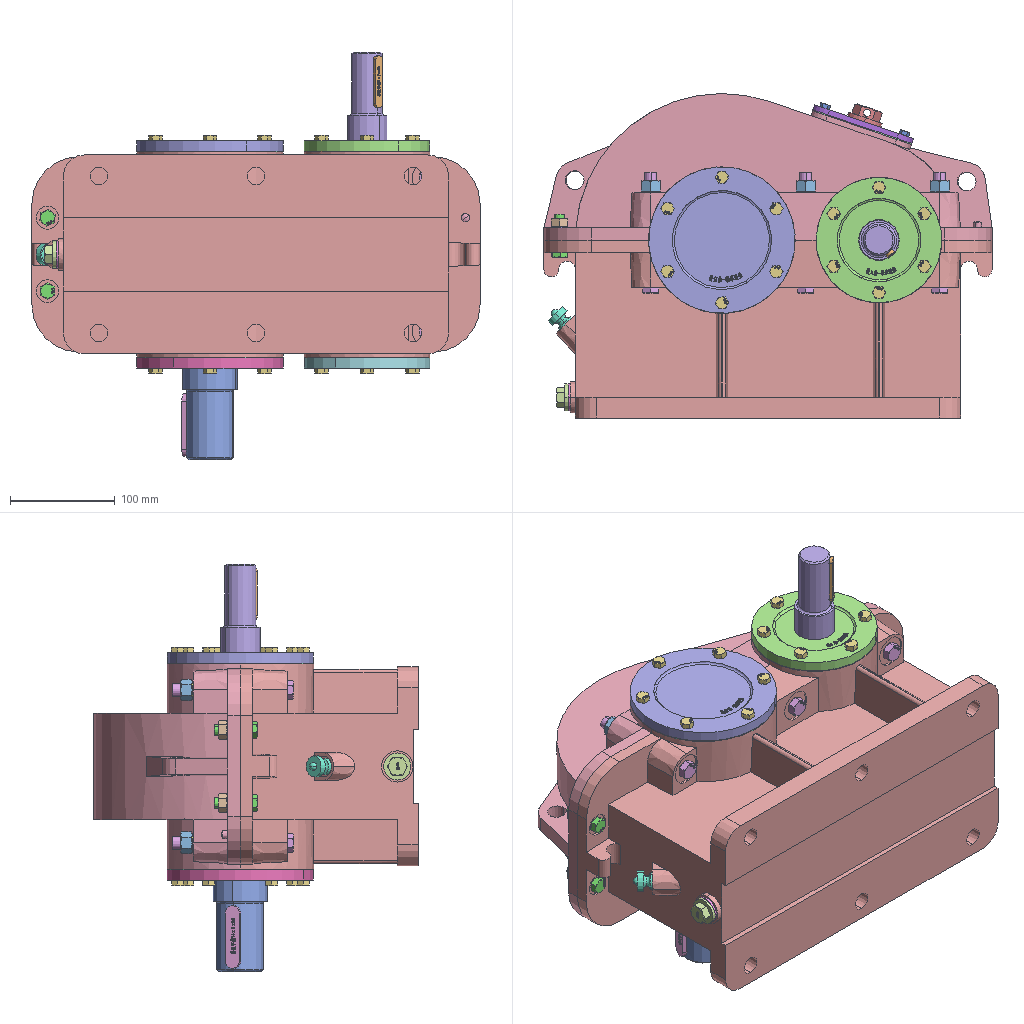Assembly | SolidWorks | 32 different items | 81 placed | box 428 x 310 x 389 mm
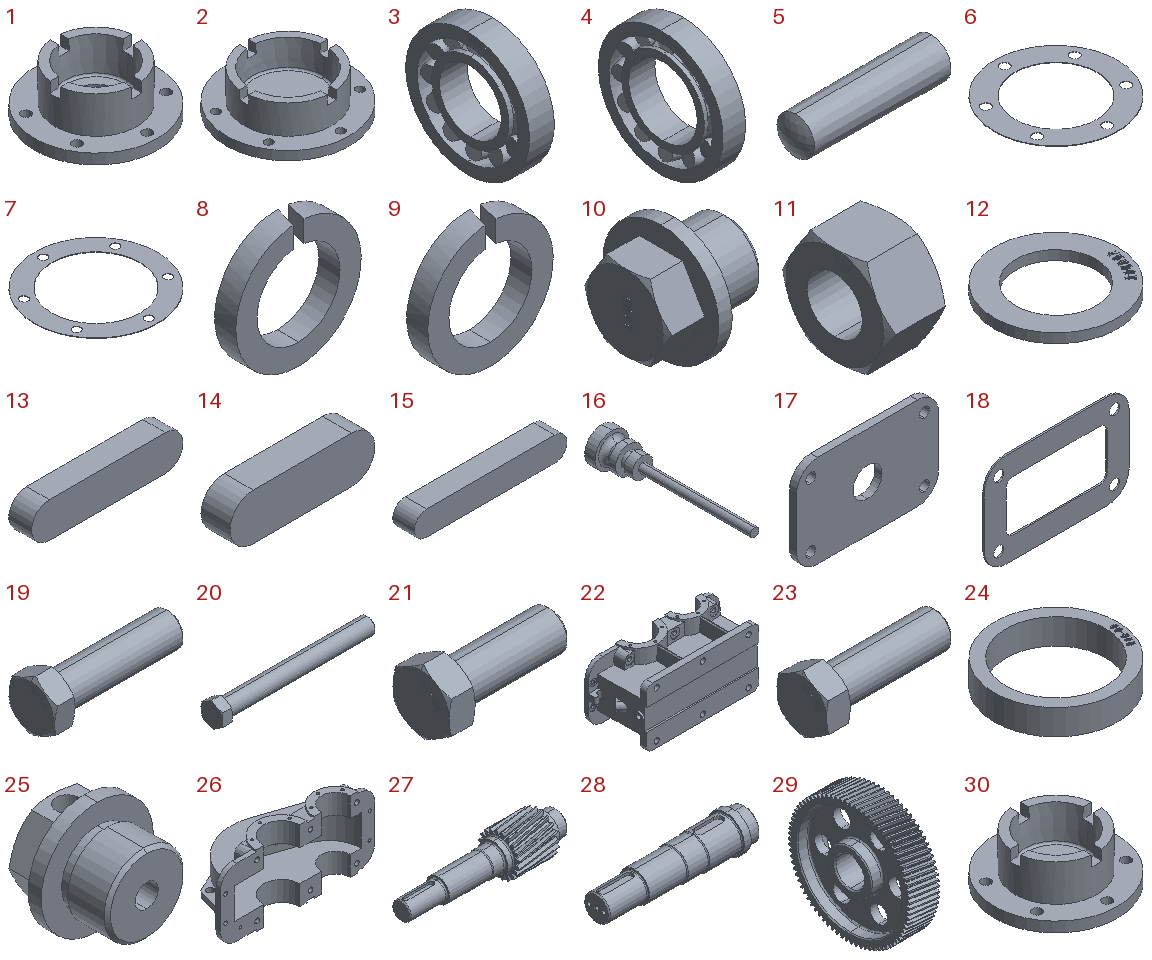Parts list (item | quantity | size | volume | features):
1 | x1 | 120 x 120 x 45.75 mm | 157075 mm3 | features ICE 6, CirPattern 2, Fillet 1, MirrorPattern 1, RevCut 1, Revolution 1
2 | x1 | 140 x 140 x 42.75 mm | 226052 mm3 | features ICE 5, CirPattern 2, Fillet 1, Revolution 1
3 | x2 | 19.75 x 80 x 80 mm | 48755 mm3 | features Revolution 5, CirPattern 1, ICE 1
4 | x2 | 22.75 x 100 x 100 mm | 79449 mm3 | features Revolution 5, CirPattern 1, ICE 1
5 | x2 | 30 x 8.048 x 8.048 mm | 1422 mm3 | features Revolution 1
6 | x2 | 120 x 120 x 0.5 mm | 2951 mm3 | features CirPattern 1, Extrusion 1, ICE 1
7 | x2 | 140 x 140 x 0.5 mm | 3579 mm3 | features CirPattern 1, Extrusion 1, ICE 1
8 | x2 | 15.4 x 2.6 x 15.4 mm | 262.555 mm3 | features ICE 2, Extrusion 1
9 | x6 | 18.4 x 3.1 x 18.4 mm | 446.274 mm3 | features ICE 2, Extrusion 1
10 | x1 | 23.1 x 26 x 26 mm | 5865 mm3 | features Chamfer 1, Extrusion 1, ICE 1, RevCut 1, Revolution 1
11 | x6 | 10.8 x 20.785 x 18 mm | 2135 mm3 | features 3DProfileFeature 1, Extrusion 1, HoleWzd 1, ICE 1, MirrorPattern 1, RevCut 1
12 | x1 | 26 x 26 x 2 mm | 607.665 mm3 | features Extrusion 1, ICE 1
13 | x1 | 60 x 9 x 14 mm | 7180 mm3 | features Extrusion 1, ICE 1
14 | x1 | 50 x 10 x 16 mm | 7451 mm3 | features Extrusion 1
15 | x1 | 50 x 7 x 8 mm | 2702 mm3 | features Extrusion 1, ICE 1
16 | x1 | 20 x 94 x 20 mm | 5502 mm3 | features Revolution 2, RevCut 1
17 | x1 | 100 x 5 x 65 mm | 29130 mm3 | features 3DProfileFeature 2, HoleWzd 2, Extrusion 1, LPattern 1
18 | x1 | 100 x 1 x 65 mm | 3724 mm3 | features 3DProfileFeature 1, Extrusion 1, HoleWzd 1, ICE 1, LPattern 1
19 | x2 | 41.4 x 14.441 x 16 mm | 3801 mm3 | features ICE 2, Chamfer 1, Extrusion 1, MirrorPattern 1, RevCut 1
20 | x6 | 115.5 x 16.057 x 18 mm | 13788 mm3 | features ICE 2, Chamfer 1, Extrusion 1, MirrorPattern 1, RevCut 1
21 | x4 | 20 x 8.68 x 10 mm | 708.376 mm3 | features ICE 2, Chamfer 1, Extrusion 1, MirrorPattern 1, RevCut 1
22 | x1 | 428 x 170 x 196 mm | 3193437 mm3 | features ICE 21, 3DProfileFeature 10, HoleWzd 10, MirrorPattern 10, Draft 8, Fillet 8, CirPattern 2, Rib 2, Extrusion 1, LPattern 1
23 | x24 | 30.3 x 11.399 x 13 mm | 1833 mm3 | features ICE 2, Chamfer 1, Extrusion 1, MirrorPattern 1, RevCut 1
24 | x1 | 68 x 68 x 14 mm | 17581 mm3 | features Extrusion 1, ICE 1
25 | x1 | 34 x 29.1 x 34 mm | 13367 mm3 | features ICE 2, RevCut 2, Chamfer 1, Extrusion 1, Revolution 1
26 | x1 | 428 x 140 x 196 mm | 1973144 mm3 | features ICE 21, 3DProfileFeature 10, HoleWzd 10, MirrorPattern 10, Draft 8, Fillet 8, CirPattern 2, Rib 2, Extrusion 1, LPattern 1
27 | x1 | 253 x 66.606 x 66.606 mm | 387584 mm3 | features ICE 4, Chamfer 2, CirPattern 1, Extrusion 1, Fillet 1, Helix 1, Revolution 1, SweepCut 1
28 | x1 | 260 x 65 x 65 mm | 565066 mm3 | features ICE 2, 3DProfileFeature 1, Chamfer 1, Fillet 1, HoleWzd 1, MirrorPattern 1, RevCut 1, Revolution 1
29 | x1 | 60 x 245.394 x 245.394 mm | 1169207 mm3 | features ICE 6, Chamfer 2, CirPattern 2, Fillet 2, 3DProfileFeature 1, Extrusion 1, Helix 1, HoleWzd 1, MirrorPattern 1, SweepCut 1
30 | x1 | 120 x 120 x 45.75 mm | 173021 mm3 | features ICE 5, CirPattern 2, Fillet 1, Revolution 1
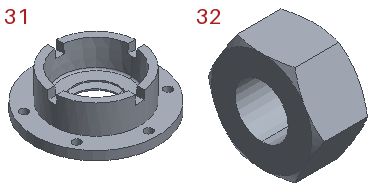31 | x1 | 140 x 140 x 42.75 mm | 195450 mm3 | features ICE 6, CirPattern 2, Fillet 1, MirrorPattern 1, RevCut 1, Revolution 1
32 | x2 | 8.4 x 18.475 x 16 mm | 1377 mm3 | features 3DProfileFeature 1, Extrusion 1, HoleWzd 1, ICE 1, MirrorPattern 1, RevCut 1
Mates (type | each side: item.copy, entity, surface, feature):
Coordinate | 22.1 select_type:25 | assembly select_type:11
Concentric | 22.1 face cylinder Cut-Extrude2 | 4.1 face cylinder Revolve1
Coincident | 22.1 face plane Cut-Extrude1 | 4.1 face plane Revolve1
Concentric | 22.1 face cylinder Cut-Extrude2 | 4.2 face cylinder Revolve1
Coincident | 22.1 face plane Cut-Extrude1 | 4.2 face plane Revolve1
Concentric | 22.1 face cylinder Cut-Extrude3 | 3.1 face cylinder Revolve1
Coincident | 22.1 face plane Cut-Extrude1 | 3.1 face plane Revolve1
Concentric | 22.1 face cylinder Cut-Extrude3 | 3.2 face cylinder Revolve1
Coincident | 22.1 face plane Cut-Extrude1 | 3.2 face plane Revolve1
Concentric | 28.1 face cylinder Revolve1 | 4.1 face cylinder Revolve1
Coincident | 28.1 face plane Revolve1 | 4.2 face plane Revolve1
Coincident | 28.1 face plane Cut-Extrude2 | 14.1 face plane Boss-Extrude1 | 2 times
Concentric | 28.1 face cylinder Cut-Extrude2 | 14.1 face cylinder Boss-Extrude1
Concentric | 28.1 face cylinder Revolve1 | 29.1 face cylinder Cut-Extrude2
Coincident | 29.1 face plane Cut-Extrude2 | 14.1 face plane Boss-Extrude1
Coincident | 28.1 face plane Revolve1 | 29.1 face plane Boss-Extrude1
Concentric | 28.1 face cylinder Revolve1 | 24.1 face cylinder Boss-Extrude1
Coincident | 29.1 face plane Boss-Extrude1 | 24.1 face plane Boss-Extrude1
Concentric | 27.1 face cylinder Revolve1 | 3.1 face cylinder Revolve1
Coincident | 27.1 face plane Revolve1 | 3.2 face plane Revolve1
Coincident | 28.1 face plane Cut-Extrude1 | 13.1 face plane Boss-Extrude1 | 2 times
Concentric | 28.1 face cylinder Cut-Extrude1 | 13.1 face cylinder Boss-Extrude1
Coincident | 15.1 face plane Boss-Extrude1 | 27.1 face plane Cut-Extrude1 | 2 times
Concentric | 15.1 face cylinder Boss-Extrude1 | 27.1 face cylinder Cut-Extrude1
GearDim | 29.1 face cylinder Boss-Extrude1 | 27.1 face cylinder Boss-Extrude1
Coincident | 22.1 face plane Cut-Extrude9 | 26.1 face plane Cut-Extrude10
Coincident | 22.1 face plane Boss-Extrude5 | 26.1 face plane Boss-Extrude5 | 2 times
Concentric | 22.1 face cylinder Mirror21 | 20.1 face cylinder Boss-Extrude2
Coincident | 22.1 face plane Mirror21 | 20.1 face plane Boss-Extrude1
Parallel | 22.1 face plane Boss-Extrude1 | 20.1 face plane Boss-Extrude1
Concentric | 9.1 face cylinder Boss-Extrude1 | 20.1 face cylinder Boss-Extrude2
PlanarAngleDim | 9.1 face plane Cut-Extrude1 | 26.1 face plane Boss-Extrude1
Coincident | 26.1 face plane Mirror21 | 9.1 face plane Boss-Extrude1
Concentric | 11.1 face cylinder M12 Tapped Hole1 | 20.1 face cylinder Boss-Extrude2
Coincident | 11.1 face plane Boss-Extrude1 | 9.1 face plane Boss-Extrude1
Parallel | 26.1 face plane Boss-Extrude5 | 11.1 face plane Boss-Extrude1
Concentric | 22.1 face cylinder Hole6 | 20.2 face cylinder Boss-Extrude2
Coincident | 22.1 face plane Mirror20 | 20.2 face plane Boss-Extrude1
Parallel | 22.1 face plane Boss-Extrude1 | 20.2 face plane Boss-Extrude1
Concentric | 9.2 face cylinder Boss-Extrude1 | 20.2 face cylinder Boss-Extrude2
PlanarAngleDim | 9.2 face plane Cut-Extrude1 | 26.1 face plane Boss-Extrude1
Coincident | 26.1 face plane Hole6 | 9.2 face plane Boss-Extrude1
Concentric | 11.2 face cylinder M12 Tapped Hole1 | 20.2 face cylinder Boss-Extrude2
Coincident | 11.2 face plane Boss-Extrude1 | 9.2 face plane Boss-Extrude1
Parallel | 26.1 face plane Boss-Extrude5 | 11.2 face plane Boss-Extrude1
Concentric | 26.1 face cylinder Mirror10 | 7.1 face cylinder Cut-Extrude1
Concentric | 22.1 face cylinder Mirror10 | 7.1 face cylinder CirPattern1
Coincident | 26.1 face plane Boss-Extrude3 | 7.1 face plane Boss-Extrude1
Concentric | 26.1 face cylinder Mirror9 | 6.1 face cylinder Cut-Extrude1
Concentric | 22.1 face cylinder Mirror9 | 6.1 face cylinder CirPattern1
Coincident | 26.1 face plane Boss-Extrude3 | 6.1 face plane Boss-Extrude1
Concentric | 26.1 face cylinder Mirror10 | 31.1 face cylinder CirPattern2
Concentric | 22.1 face cylinder Mirror10 | 31.1 face cylinder CirPattern2
Coincident | 7.1 face plane Boss-Extrude1 | 31.1 face plane Revolve1
Concentric | 26.1 face cylinder Mirror9 | 30.1 face cylinder CirPattern2
Concentric | 22.1 face cylinder Mirror9 | 30.1 face cylinder CirPattern2
Coincident | 6.1 face plane Boss-Extrude1 | 30.1 face plane Revolve1
Concentric | 26.1 face cylinder M8 Tapped Hole1 | 2.1 face cylinder CirPattern2
Concentric | 22.1 face cylinder CirPattern1 | 2.1 face cylinder CirPattern2
Coincident | 7.2 face plane Boss-Extrude1 | 2.1 face plane Revolve1
Concentric | 26.1 face cylinder M8 Tapped Hole2 | 1.1 face cylinder CirPattern2
Concentric | 22.1 face cylinder CirPattern2 | 1.1 face cylinder CirPattern2
Coincident | 6.2 face plane Boss-Extrude1 | 1.1 face plane Revolve1
Concentric | 31.1 face cylinder CirPattern2 | 23.1 face cylinder Boss-Extrude2
Coincident | 31.1 face plane Revolve1 | 23.1 face plane Boss-Extrude1
Parallel | 22.1 face plane Boss-Extrude6 | 23.1 face plane Boss-Extrude1
Coincident | 26.1 face plane Boss-Extrude12 | 18.1 face plane Boss-Extrude1 | 3 times
Coincident | 17.1 face plane Boss-Extrude1 | 18.1 face plane Boss-Extrude1
Coincident | 26.1 face plane Boss-Extrude12 | 17.1 face plane Boss-Extrude1 | 2 times
Concentric | 17.1 face cylinder M24 Tapped Hole2 | 25.1 face cylinder Revolve1
Coincident | 17.1 face plane Boss-Extrude1 | 25.1 face plane Revolve1
Parallel | 17.1 face plane Boss-Extrude1 | 25.1 face plane Boss-Extrude1
Concentric | 17.1 face cylinder LPattern1 | 21.1 face cylinder Boss-Extrude2
Coincident | 17.1 face plane Boss-Extrude1 | 21.1 face plane Boss-Extrude1
Parallel | 26.1 face plane Boss-Extrude12 | 21.1 face plane Boss-Extrude1
Concentric | 22.1 face cylinder M16x1.5 Tapped Hole1 | 12.1 face cylinder Boss-Extrude1
Coincident | 22.1 face plane Boss-Extrude7 | 12.1 face plane Boss-Extrude1
Concentric | 22.1 face cylinder M16x1.5 Tapped Hole1 | 10.1 face cylinder Revolve1
Coincident | 10.1 face plane Revolve1 | 12.1 face plane Boss-Extrude1
Parallel | 22.1 face plane Boss-Extrude6 | 10.1 face plane Boss-Extrude1
Concentric | 22.1 face cylinder M12 Tapped Hole1 | 16.1 face cylinder Revolve1
Coincident | 22.1 face plane Cut-Extrude5 | 16.1 face plane Revolve1
Concentric | 22.1 face cylinder Hole7 | 19.1 face cylinder Boss-Extrude2
Coincident | 22.1 face plane Mirror22 | 19.1 face plane Boss-Extrude1
Parallel | 22.1 face plane Boss-Extrude5 | 19.1 face plane Boss-Extrude1
Concentric | 8.1 face cylinder Boss-Extrude1 | 19.1 face cylinder Boss-Extrude2
PlanarAngleDim | 8.1 face plane Cut-Extrude1 | 26.1 face plane Boss-Extrude10
Coincident | 26.1 face plane Hole7 | 8.1 face plane Boss-Extrude1
Concentric | 32.1 face cylinder M10 Tapped Hole1 | 19.1 face cylinder Boss-Extrude2
Coincident | 32.1 face plane Boss-Extrude1 | 8.1 face plane Boss-Extrude1
Parallel | 26.1 face plane Boss-Extrude5 | 32.1 face plane Boss-Extrude1
Concentric | 26.1 face cylinder Cut-Extrude4 | 5.1 face cone Revolve1
Tangent | 22.1 face plane Mirror2 | 5.1 face sphere Revolve1
Concentric | 26.1 face cylinder Cut-Extrude4 | 5.2 face cone Revolve1
Tangent | 22.1 face plane Mirror2 | 5.2 face sphere Revolve1
Concentric | 1.1 face cylinder CirPattern2 | 23.2 face cylinder Boss-Extrude2
Coincident | 1.1 face plane Revolve1 | 23.2 face plane Boss-Extrude1
Parallel | 22.1 face plane Boss-Extrude6 | 23.2 face plane Boss-Extrude1